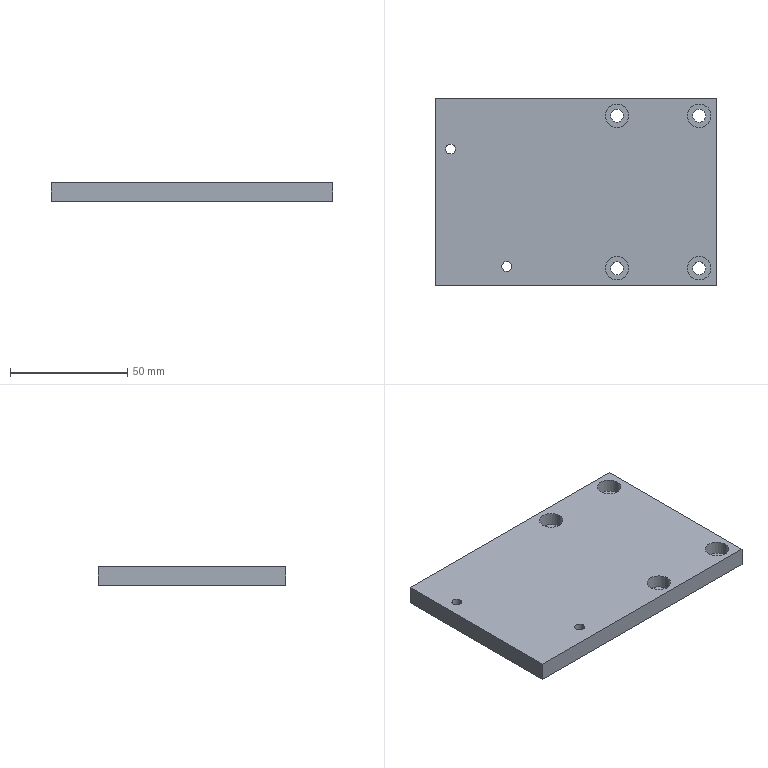Part | STEP file | X77-07006 | 1 solid | 30 faces | box 120 x 80 x 8 mm | volume 74569 mm3 | cylinder 20 | plane 10 | commonest cylinder face diameters 5.5 x8 10 x8 4.2 x4
STEP:
#1=CARTESIAN_POINT('',(-295.5,1019.962,2.3));
#2=VERTEX_POINT('',#1);
#3=CARTESIAN_POINT('',(-285.5,1019.962,2.3));
#4=VERTEX_POINT('',#3);
#5=CARTESIAN_POINT('',(-290.5,1019.962,2.3));
#6=DIRECTION('',(0.,0.,1.));
#7=DIRECTION('',(1.,0.,0.));
#8=AXIS2_PLACEMENT_3D('',#5,#6,#7);
#9=CIRCLE('',#8,5.);
#10=EDGE_CURVE('',#2,#4,#9,.T.);
#11=ORIENTED_EDGE('',*,*,#10,.F.);
#12=CARTESIAN_POINT('',(-295.5,1019.962,8.));
#13=VERTEX_POINT('',#12);
#14=CARTESIAN_POINT('',(-295.5,1019.962,8.));
#15=DIRECTION('',(0.,0.,1.));
#16=VECTOR('',#15,1000.);
#17=LINE('',#14,#16);
#18=EDGE_CURVE('',#2,#13,#17,.T.);
#19=ORIENTED_EDGE('',*,*,#18,.T.);
#20=CARTESIAN_POINT('',(-285.5,1019.962,8.));
#21=VERTEX_POINT('',#20);
#22=CARTESIAN_POINT('',(-290.5,1019.962,8.));
#23=DIRECTION('',(0.,0.,1.));
#24=DIRECTION('',(1.,0.,0.));
#25=AXIS2_PLACEMENT_3D('',#22,#23,#24);
#26=CIRCLE('',#25,5.);
#27=EDGE_CURVE('',#13,#21,#26,.T.);
#28=ORIENTED_EDGE('',*,*,#27,.T.);
#29=CARTESIAN_POINT('',(-285.5,1019.962,8.));
#30=DIRECTION('',(0.,0.,1.));
#31=VECTOR('',#30,1000.);
#32=LINE('',#29,#31);
#33=EDGE_CURVE('',#4,#21,#32,.T.);
#34=ORIENTED_EDGE('',*,*,#33,.F.);
#35=EDGE_LOOP('',(#11,#19,#28,#34));
#36=FACE_OUTER_BOUND('',#35,.T.);
#37=CARTESIAN_POINT('',(-290.5,1019.962,8.));
#38=DIRECTION('',(0.,0.,1.));
#39=DIRECTION('',(1.,0.,0.));
#40=AXIS2_PLACEMENT_3D('',#37,#38,#39);
#41=CYLINDRICAL_SURFACE('',#40,5.);
#42=ADVANCED_FACE('',(#36),#41,.F.);
#43=CARTESIAN_POINT('',(-293.25,1019.962,0.));
#44=VERTEX_POINT('',#43);
#45=CARTESIAN_POINT('',(-287.75,1019.962,0.));
#46=VERTEX_POINT('',#45);
#47=CARTESIAN_POINT('',(-290.5,1019.962,0.));
#48=DIRECTION('',(0.,0.,1.));
#49=DIRECTION('',(1.,0.,0.));
#50=AXIS2_PLACEMENT_3D('',#47,#48,#49);
#51=CIRCLE('',#50,2.75);
#52=EDGE_CURVE('',#44,#46,#51,.T.);
#53=ORIENTED_EDGE('',*,*,#52,.F.);
#54=CARTESIAN_POINT('',(-293.25,1019.962,2.3));
#55=VERTEX_POINT('',#54);
#56=CARTESIAN_POINT('',(-293.25,1019.962,8.));
#57=DIRECTION('',(0.,0.,1.));
#58=VECTOR('',#57,1000.);
#59=LINE('',#56,#58);
#60=EDGE_CURVE('',#44,#55,#59,.T.);
#61=ORIENTED_EDGE('',*,*,#60,.T.);
#62=CARTESIAN_POINT('',(-287.75,1019.962,2.3));
#63=VERTEX_POINT('',#62);
#64=CARTESIAN_POINT('',(-290.5,1019.962,2.3));
#65=DIRECTION('',(0.,0.,1.));
#66=DIRECTION('',(1.,0.,0.));
#67=AXIS2_PLACEMENT_3D('',#64,#65,#66);
#68=CIRCLE('',#67,2.75);
#69=EDGE_CURVE('',#55,#63,#68,.T.);
#70=ORIENTED_EDGE('',*,*,#69,.T.);
#71=CARTESIAN_POINT('',(-287.75,1019.962,8.));
#72=DIRECTION('',(0.,0.,1.));
#73=VECTOR('',#72,1000.);
#74=LINE('',#71,#73);
#75=EDGE_CURVE('',#46,#63,#74,.T.);
#76=ORIENTED_EDGE('',*,*,#75,.F.);
#77=EDGE_LOOP('',(#53,#61,#70,#76));
#78=FACE_OUTER_BOUND('',#77,.T.);
#79=CARTESIAN_POINT('',(-290.5,1019.962,8.));
#80=DIRECTION('',(0.,0.,1.));
#81=DIRECTION('',(1.,0.,0.));
#82=AXIS2_PLACEMENT_3D('',#79,#80,#81);
#83=CYLINDRICAL_SURFACE('',#82,2.75);
#84=ADVANCED_FACE('',(#78),#83,.F.);
#85=CARTESIAN_POINT('',(-260.5,1019.962,2.3));
#86=VERTEX_POINT('',#85);
#87=CARTESIAN_POINT('',(-250.5,1019.962,2.3));
#88=VERTEX_POINT('',#87);
#89=CARTESIAN_POINT('',(-255.5,1019.962,2.3));
#90=DIRECTION('',(0.,0.,1.));
#91=DIRECTION('',(1.,0.,0.));
#92=AXIS2_PLACEMENT_3D('',#89,#90,#91);
#93=CIRCLE('',#92,5.);
#94=EDGE_CURVE('',#86,#88,#93,.T.);
#95=ORIENTED_EDGE('',*,*,#94,.F.);
#96=CARTESIAN_POINT('',(-260.5,1019.962,8.));
#97=VERTEX_POINT('',#96);
#98=CARTESIAN_POINT('',(-260.5,1019.962,8.));
#99=DIRECTION('',(0.,0.,1.));
#100=VECTOR('',#99,1000.);
#101=LINE('',#98,#100);
#102=EDGE_CURVE('',#86,#97,#101,.T.);
#103=ORIENTED_EDGE('',*,*,#102,.T.);
#104=CARTESIAN_POINT('',(-250.5,1019.962,8.));
#105=VERTEX_POINT('',#104);
#106=CARTESIAN_POINT('',(-255.5,1019.962,8.));
#107=DIRECTION('',(0.,0.,1.));
#108=DIRECTION('',(1.,0.,0.));
#109=AXIS2_PLACEMENT_3D('',#106,#107,#108);
#110=CIRCLE('',#109,5.);
#111=EDGE_CURVE('',#97,#105,#110,.T.);
#112=ORIENTED_EDGE('',*,*,#111,.T.);
#113=CARTESIAN_POINT('',(-250.5,1019.962,8.));
#114=DIRECTION('',(0.,0.,1.));
#115=VECTOR('',#114,1000.);
#116=LINE('',#113,#115);
#117=EDGE_CURVE('',#88,#105,#116,.T.);
#118=ORIENTED_EDGE('',*,*,#117,.F.);
#119=EDGE_LOOP('',(#95,#103,#112,#118));
#120=FACE_OUTER_BOUND('',#119,.T.);
#121=CARTESIAN_POINT('',(-255.5,1019.962,8.));
#122=DIRECTION('',(0.,0.,1.));
#123=DIRECTION('',(1.,0.,0.));
#124=AXIS2_PLACEMENT_3D('',#121,#122,#123);
#125=CYLINDRICAL_SURFACE('',#124,5.);
#126=ADVANCED_FACE('',(#120),#125,.F.);
#127=CARTESIAN_POINT('',(-258.25,1019.962,0.));
#128=VERTEX_POINT('',#127);
#129=CARTESIAN_POINT('',(-252.75,1019.962,0.));
#130=VERTEX_POINT('',#129);
#131=CARTESIAN_POINT('',(-255.5,1019.962,0.));
#132=DIRECTION('',(0.,0.,1.));
#133=DIRECTION('',(1.,0.,0.));
#134=AXIS2_PLACEMENT_3D('',#131,#132,#133);
#135=CIRCLE('',#134,2.75);
#136=EDGE_CURVE('',#128,#130,#135,.T.);
#137=ORIENTED_EDGE('',*,*,#136,.F.);
#138=CARTESIAN_POINT('',(-258.25,1019.962,2.3));
#139=VERTEX_POINT('',#138);
#140=CARTESIAN_POINT('',(-258.25,1019.962,8.));
#141=DIRECTION('',(0.,0.,1.));
#142=VECTOR('',#141,1000.);
#143=LINE('',#140,#142);
#144=EDGE_CURVE('',#128,#139,#143,.T.);
#145=ORIENTED_EDGE('',*,*,#144,.T.);
#146=CARTESIAN_POINT('',(-252.75,1019.962,2.3));
#147=VERTEX_POINT('',#146);
#148=CARTESIAN_POINT('',(-255.5,1019.962,2.3));
#149=DIRECTION('',(0.,0.,1.));
#150=DIRECTION('',(1.,0.,0.));
#151=AXIS2_PLACEMENT_3D('',#148,#149,#150);
#152=CIRCLE('',#151,2.75);
#153=EDGE_CURVE('',#139,#147,#152,.T.);
#154=ORIENTED_EDGE('',*,*,#153,.T.);
#155=CARTESIAN_POINT('',(-252.75,1019.962,8.));
#156=DIRECTION('',(0.,0.,1.));
#157=VECTOR('',#156,1000.);
#158=LINE('',#155,#157);
#159=EDGE_CURVE('',#130,#147,#158,.T.);
#160=ORIENTED_EDGE('',*,*,#159,.F.);
#161=EDGE_LOOP('',(#137,#145,#154,#160));
#162=FACE_OUTER_BOUND('',#161,.T.);
#163=CARTESIAN_POINT('',(-255.5,1019.962,8.));
#164=DIRECTION('',(0.,0.,1.));
#165=DIRECTION('',(1.,0.,0.));
#166=AXIS2_PLACEMENT_3D('',#163,#164,#165);
#167=CYLINDRICAL_SURFACE('',#166,2.75);
#168=ADVANCED_FACE('',(#162),#167,.F.);
#169=CARTESIAN_POINT('',(-295.5,954.962,2.3));
#170=VERTEX_POINT('',#169);
#171=CARTESIAN_POINT('',(-285.5,954.962,2.3));
#172=VERTEX_POINT('',#171);
#173=CARTESIAN_POINT('',(-290.5,954.962,2.3));
#174=DIRECTION('',(0.,0.,1.));
#175=DIRECTION('',(1.,0.,0.));
#176=AXIS2_PLACEMENT_3D('',#173,#174,#175);
#177=CIRCLE('',#176,5.);
#178=EDGE_CURVE('',#170,#172,#177,.T.);
#179=ORIENTED_EDGE('',*,*,#178,.F.);
#180=CARTESIAN_POINT('',(-295.5,954.962,8.));
#181=VERTEX_POINT('',#180);
#182=CARTESIAN_POINT('',(-295.5,954.962,8.));
#183=DIRECTION('',(0.,0.,1.));
#184=VECTOR('',#183,1000.);
#185=LINE('',#182,#184);
#186=EDGE_CURVE('',#170,#181,#185,.T.);
#187=ORIENTED_EDGE('',*,*,#186,.T.);
#188=CARTESIAN_POINT('',(-285.5,954.962,8.));
#189=VERTEX_POINT('',#188);
#190=CARTESIAN_POINT('',(-290.5,954.962,8.));
#191=DIRECTION('',(0.,0.,1.));
#192=DIRECTION('',(1.,0.,0.));
#193=AXIS2_PLACEMENT_3D('',#190,#191,#192);
#194=CIRCLE('',#193,5.);
#195=EDGE_CURVE('',#181,#189,#194,.T.);
#196=ORIENTED_EDGE('',*,*,#195,.T.);
#197=CARTESIAN_POINT('',(-285.5,954.962,8.));
#198=DIRECTION('',(0.,0.,1.));
#199=VECTOR('',#198,1000.);
#200=LINE('',#197,#199);
#201=EDGE_CURVE('',#172,#189,#200,.T.);
#202=ORIENTED_EDGE('',*,*,#201,.F.);
#203=EDGE_LOOP('',(#179,#187,#196,#202));
#204=FACE_OUTER_BOUND('',#203,.T.);
#205=CARTESIAN_POINT('',(-290.5,954.962,8.));
#206=DIRECTION('',(0.,0.,1.));
#207=DIRECTION('',(1.,0.,0.));
#208=AXIS2_PLACEMENT_3D('',#205,#206,#207);
#209=CYLINDRICAL_SURFACE('',#208,5.);
#210=ADVANCED_FACE('',(#204),#209,.F.);
#211=CARTESIAN_POINT('',(-293.25,954.962,0.));
#212=VERTEX_POINT('',#211);
#213=CARTESIAN_POINT('',(-287.75,954.962,0.));
#214=VERTEX_POINT('',#213);
#215=CARTESIAN_POINT('',(-290.5,954.962,0.));
#216=DIRECTION('',(0.,0.,1.));
#217=DIRECTION('',(1.,0.,0.));
#218=AXIS2_PLACEMENT_3D('',#215,#216,#217);
#219=CIRCLE('',#218,2.75);
#220=EDGE_CURVE('',#212,#214,#219,.T.);
#221=ORIENTED_EDGE('',*,*,#220,.F.);
#222=CARTESIAN_POINT('',(-293.25,954.962,2.3));
#223=VERTEX_POINT('',#222);
#224=CARTESIAN_POINT('',(-293.25,954.962,8.));
#225=DIRECTION('',(0.,0.,1.));
#226=VECTOR('',#225,1000.);
#227=LINE('',#224,#226);
#228=EDGE_CURVE('',#212,#223,#227,.T.);
#229=ORIENTED_EDGE('',*,*,#228,.T.);
#230=CARTESIAN_POINT('',(-287.75,954.962,2.3));
#231=VERTEX_POINT('',#230);
#232=CARTESIAN_POINT('',(-290.5,954.962,2.3));
#233=DIRECTION('',(0.,0.,1.));
#234=DIRECTION('',(1.,0.,0.));
#235=AXIS2_PLACEMENT_3D('',#232,#233,#234);
#236=CIRCLE('',#235,2.75);
#237=EDGE_CURVE('',#223,#231,#236,.T.);
#238=ORIENTED_EDGE('',*,*,#237,.T.);
#239=CARTESIAN_POINT('',(-287.75,954.962,8.));
#240=DIRECTION('',(0.,0.,1.));
#241=VECTOR('',#240,1000.);
#242=LINE('',#239,#241);
#243=EDGE_CURVE('',#214,#231,#242,.T.);
#244=ORIENTED_EDGE('',*,*,#243,.F.);
#245=EDGE_LOOP('',(#221,#229,#238,#244));
#246=FACE_OUTER_BOUND('',#245,.T.);
#247=CARTESIAN_POINT('',(-290.5,954.962,8.));
#248=DIRECTION('',(0.,0.,1.));
#249=DIRECTION('',(1.,0.,0.));
#250=AXIS2_PLACEMENT_3D('',#247,#248,#249);
#251=CYLINDRICAL_SURFACE('',#250,2.75);
#252=ADVANCED_FACE('',(#246),#251,.F.);
#253=CARTESIAN_POINT('',(-260.5,954.962,2.3));
#254=VERTEX_POINT('',#253);
#255=CARTESIAN_POINT('',(-250.5,954.962,2.3));
#256=VERTEX_POINT('',#255);
#257=CARTESIAN_POINT('',(-255.5,954.962,2.3));
#258=DIRECTION('',(0.,0.,1.));
#259=DIRECTION('',(1.,0.,0.));
#260=AXIS2_PLACEMENT_3D('',#257,#258,#259);
#261=CIRCLE('',#260,5.);
#262=EDGE_CURVE('',#254,#256,#261,.T.);
#263=ORIENTED_EDGE('',*,*,#262,.F.);
#264=CARTESIAN_POINT('',(-260.5,954.962,8.));
#265=VERTEX_POINT('',#264);
#266=CARTESIAN_POINT('',(-260.5,954.962,8.));
#267=DIRECTION('',(0.,0.,1.));
#268=VECTOR('',#267,1000.);
#269=LINE('',#266,#268);
#270=EDGE_CURVE('',#254,#265,#269,.T.);
#271=ORIENTED_EDGE('',*,*,#270,.T.);
#272=CARTESIAN_POINT('',(-250.5,954.962,8.));
#273=VERTEX_POINT('',#272);
#274=CARTESIAN_POINT('',(-255.5,954.962,8.));
#275=DIRECTION('',(0.,0.,1.));
#276=DIRECTION('',(1.,0.,0.));
#277=AXIS2_PLACEMENT_3D('',#274,#275,#276);
#278=CIRCLE('',#277,5.);
#279=EDGE_CURVE('',#265,#273,#278,.T.);
#280=ORIENTED_EDGE('',*,*,#279,.T.);
#281=CARTESIAN_POINT('',(-250.5,954.962,8.));
#282=DIRECTION('',(0.,0.,1.));
#283=VECTOR('',#282,1000.);
#284=LINE('',#281,#283);
#285=EDGE_CURVE('',#256,#273,#284,.T.);
#286=ORIENTED_EDGE('',*,*,#285,.F.);
#287=EDGE_LOOP('',(#263,#271,#280,#286));
#288=FACE_OUTER_BOUND('',#287,.T.);
#289=CARTESIAN_POINT('',(-255.5,954.962,8.));
#290=DIRECTION('',(0.,0.,1.));
#291=DIRECTION('',(1.,0.,0.));
#292=AXIS2_PLACEMENT_3D('',#289,#290,#291);
#293=CYLINDRICAL_SURFACE('',#292,5.);
#294=ADVANCED_FACE('',(#288),#293,.F.);
#295=CARTESIAN_POINT('',(-258.25,954.962,0.));
#296=VERTEX_POINT('',#295);
#297=CARTESIAN_POINT('',(-252.75,954.962,0.));
#298=VERTEX_POINT('',#297);
#299=CARTESIAN_POINT('',(-255.5,954.962,0.));
#300=DIRECTION('',(0.,0.,1.));
#301=DIRECTION('',(1.,0.,0.));
#302=AXIS2_PLACEMENT_3D('',#299,#300,#301);
#303=CIRCLE('',#302,2.75);
#304=EDGE_CURVE('',#296,#298,#303,.T.);
#305=ORIENTED_EDGE('',*,*,#304,.F.);
#306=CARTESIAN_POINT('',(-258.25,954.962,2.3));
#307=VERTEX_POINT('',#306);
#308=CARTESIAN_POINT('',(-258.25,954.962,8.));
#309=DIRECTION('',(0.,0.,1.));
#310=VECTOR('',#309,1000.);
#311=LINE('',#308,#310);
#312=EDGE_CURVE('',#296,#307,#311,.T.);
#313=ORIENTED_EDGE('',*,*,#312,.T.);
#314=CARTESIAN_POINT('',(-252.75,954.962,2.3));
#315=VERTEX_POINT('',#314);
#316=CARTESIAN_POINT('',(-255.5,954.962,2.3));
#317=DIRECTION('',(0.,0.,1.));
#318=DIRECTION('',(1.,0.,0.));
#319=AXIS2_PLACEMENT_3D('',#316,#317,#318);
#320=CIRCLE('',#319,2.75);
#321=EDGE_CURVE('',#307,#315,#320,.T.);
#322=ORIENTED_EDGE('',*,*,#321,.T.);
#323=CARTESIAN_POINT('',(-252.75,954.962,8.));
#324=DIRECTION('',(0.,0.,1.));
#325=VECTOR('',#324,1000.);
#326=LINE('',#323,#325);
#327=EDGE_CURVE('',#298,#315,#326,.T.);
#328=ORIENTED_EDGE('',*,*,#327,.F.);
#329=EDGE_LOOP('',(#305,#313,#322,#328));
#330=FACE_OUTER_BOUND('',#329,.T.);
#331=CARTESIAN_POINT('',(-255.5,954.962,8.));
#332=DIRECTION('',(0.,0.,1.));
#333=DIRECTION('',(1.,0.,0.));
#334=AXIS2_PLACEMENT_3D('',#331,#332,#333);
#335=CYLINDRICAL_SURFACE('',#334,2.75);
#336=ADVANCED_FACE('',(#330),#335,.F.);
#337=CARTESIAN_POINT('',(-339.6,955.739,8.));
#338=VERTEX_POINT('',#337);
#339=CARTESIAN_POINT('',(-335.4,955.739,8.));
#340=VERTEX_POINT('',#339);
#341=CARTESIAN_POINT('',(-337.5,955.739,8.));
#342=DIRECTION('',(0.,0.,1.));
#343=DIRECTION('',(1.,0.,0.));
#344=AXIS2_PLACEMENT_3D('',#341,#342,#343);
#345=CIRCLE('',#344,2.1);
#346=EDGE_CURVE('',#338,#340,#345,.T.);
#347=ORIENTED_EDGE('',*,*,#346,.T.);
#348=CARTESIAN_POINT('',(-335.4,955.739,0.));
#349=VERTEX_POINT('',#348);
#350=CARTESIAN_POINT('',(-335.4,955.739,0.));
#351=DIRECTION('',(0.,0.,-1.));
#352=VECTOR('',#351,1000.);
#353=LINE('',#350,#352);
#354=EDGE_CURVE('',#340,#349,#353,.T.);
#355=ORIENTED_EDGE('',*,*,#354,.T.);
#356=CARTESIAN_POINT('',(-339.6,955.739,0.));
#357=VERTEX_POINT('',#356);
#358=CARTESIAN_POINT('',(-337.5,955.739,0.));
#359=DIRECTION('',(0.,0.,-1.));
#360=DIRECTION('',(-1.,0.,0.));
#361=AXIS2_PLACEMENT_3D('',#358,#359,#360);
#362=CIRCLE('',#361,2.1);
#363=EDGE_CURVE('',#349,#357,#362,.T.);
#364=ORIENTED_EDGE('',*,*,#363,.T.);
#365=CARTESIAN_POINT('',(-339.6,955.739,0.));
#366=DIRECTION('',(0.,0.,-1.));
#367=VECTOR('',#366,1000.);
#368=LINE('',#365,#367);
#369=EDGE_CURVE('',#338,#357,#368,.T.);
#370=ORIENTED_EDGE('',*,*,#369,.F.);
#371=EDGE_LOOP('',(#347,#355,#364,#370));
#372=FACE_OUTER_BOUND('',#371,.T.);
#373=CARTESIAN_POINT('',(-337.5,955.739,0.));
#374=DIRECTION('',(0.,0.,-1.));
#375=DIRECTION('',(-1.,0.,0.));
#376=AXIS2_PLACEMENT_3D('',#373,#374,#375);
#377=CYLINDRICAL_SURFACE('',#376,2.1);
#378=ADVANCED_FACE('',(#372),#377,.F.);
#379=CARTESIAN_POINT('',(-363.6,1005.739,8.));
#380=VERTEX_POINT('',#379);
#381=CARTESIAN_POINT('',(-359.4,1005.739,8.));
#382=VERTEX_POINT('',#381);
#383=CARTESIAN_POINT('',(-361.5,1005.739,8.));
#384=DIRECTION('',(0.,0.,1.));
#385=DIRECTION('',(1.,0.,0.));
#386=AXIS2_PLACEMENT_3D('',#383,#384,#385);
#387=CIRCLE('',#386,2.1);
#388=EDGE_CURVE('',#380,#382,#387,.T.);
#389=ORIENTED_EDGE('',*,*,#388,.T.);
#390=CARTESIAN_POINT('',(-359.4,1005.739,0.));
#391=VERTEX_POINT('',#390);
#392=CARTESIAN_POINT('',(-359.4,1005.739,0.));
#393=DIRECTION('',(0.,0.,-1.));
#394=VECTOR('',#393,1000.);
#395=LINE('',#392,#394);
#396=EDGE_CURVE('',#382,#391,#395,.T.);
#397=ORIENTED_EDGE('',*,*,#396,.T.);
#398=CARTESIAN_POINT('',(-363.6,1005.739,0.));
#399=VERTEX_POINT('',#398);
#400=CARTESIAN_POINT('',(-361.5,1005.739,0.));
#401=DIRECTION('',(0.,0.,-1.));
#402=DIRECTION('',(-1.,0.,0.));
#403=AXIS2_PLACEMENT_3D('',#400,#401,#402);
#404=CIRCLE('',#403,2.1);
#405=EDGE_CURVE('',#391,#399,#404,.T.);
#406=ORIENTED_EDGE('',*,*,#405,.T.);
#407=CARTESIAN_POINT('',(-363.6,1005.739,0.));
#408=DIRECTION('',(0.,0.,-1.));
#409=VECTOR('',#408,1000.);
#410=LINE('',#407,#409);
#411=EDGE_CURVE('',#380,#399,#410,.T.);
#412=ORIENTED_EDGE('',*,*,#411,.F.);
#413=EDGE_LOOP('',(#389,#397,#406,#412));
#414=FACE_OUTER_BOUND('',#413,.T.);
#415=CARTESIAN_POINT('',(-361.5,1005.739,0.));
#416=DIRECTION('',(0.,0.,-1.));
#417=DIRECTION('',(-1.,0.,0.));
#418=AXIS2_PLACEMENT_3D('',#415,#416,#417);
#419=CYLINDRICAL_SURFACE('',#418,2.1);
#420=ADVANCED_FACE('',(#414),#419,.F.);
#421=CARTESIAN_POINT('',(-368.,1027.462,0.));
#422=VERTEX_POINT('',#421);
#423=CARTESIAN_POINT('',(-368.,947.462,0.));
#424=VERTEX_POINT('',#423);
#425=CARTESIAN_POINT('',(-368.,1027.462,0.));
#426=DIRECTION('',(0.,-1.,0.));
#427=VECTOR('',#426,1000.);
#428=LINE('',#425,#427);
#429=EDGE_CURVE('',#422,#424,#428,.T.);
#430=ORIENTED_EDGE('',*,*,#429,.T.);
#431=CARTESIAN_POINT('',(-368.,947.462,8.));
#432=VERTEX_POINT('',#431);
#433=CARTESIAN_POINT('',(-368.,947.462,8.));
#434=DIRECTION('',(0.,0.,-1.));
#435=VECTOR('',#434,1000.);
#436=LINE('',#433,#435);
#437=EDGE_CURVE('',#432,#424,#436,.T.);
#438=ORIENTED_EDGE('',*,*,#437,.F.);
#439=CARTESIAN_POINT('',(-368.,1027.462,8.));
#440=VERTEX_POINT('',#439);
#441=CARTESIAN_POINT('',(-368.,1027.462,8.));
#442=DIRECTION('',(0.,-1.,0.));
#443=VECTOR('',#442,1000.);
#444=LINE('',#441,#443);
#445=EDGE_CURVE('',#440,#432,#444,.T.);
#446=ORIENTED_EDGE('',*,*,#445,.F.);
#447=CARTESIAN_POINT('',(-368.,1027.462,8.));
#448=DIRECTION('',(0.,0.,-1.));
#449=VECTOR('',#448,1000.);
#450=LINE('',#447,#449);
#451=EDGE_CURVE('',#440,#422,#450,.T.);
#452=ORIENTED_EDGE('',*,*,#451,.T.);
#453=EDGE_LOOP('',(#430,#438,#446,#452));
#454=FACE_OUTER_BOUND('',#453,.T.);
#455=CARTESIAN_POINT('',(-368.,1027.462,8.));
#456=DIRECTION('',(1.,0.,0.));
#457=DIRECTION('',(0.,0.,-1.));
#458=AXIS2_PLACEMENT_3D('',#455,#456,#457);
#459=PLANE('',#458);
#460=ADVANCED_FACE('',(#454),#459,.F.);
#461=CARTESIAN_POINT('',(-248.,947.462,0.));
#462=VERTEX_POINT('',#461);
#463=CARTESIAN_POINT('',(-368.,947.462,0.));
#464=DIRECTION('',(1.,0.,0.));
#465=VECTOR('',#464,1000.);
#466=LINE('',#463,#465);
#467=EDGE_CURVE('',#424,#462,#466,.T.);
#468=ORIENTED_EDGE('',*,*,#467,.T.);
#469=CARTESIAN_POINT('',(-248.,947.462,8.));
#470=VERTEX_POINT('',#469);
#471=CARTESIAN_POINT('',(-248.,947.462,8.));
#472=DIRECTION('',(0.,0.,-1.));
#473=VECTOR('',#472,1000.);
#474=LINE('',#471,#473);
#475=EDGE_CURVE('',#470,#462,#474,.T.);
#476=ORIENTED_EDGE('',*,*,#475,.F.);
#477=CARTESIAN_POINT('',(-368.,947.462,8.));
#478=DIRECTION('',(1.,0.,0.));
#479=VECTOR('',#478,1000.);
#480=LINE('',#477,#479);
#481=EDGE_CURVE('',#432,#470,#480,.T.);
#482=ORIENTED_EDGE('',*,*,#481,.F.);
#483=ORIENTED_EDGE('',*,*,#437,.T.);
#484=EDGE_LOOP('',(#468,#476,#482,#483));
#485=FACE_OUTER_BOUND('',#484,.T.);
#486=CARTESIAN_POINT('',(-368.,947.462,8.));
#487=DIRECTION('',(0.,1.,0.));
#488=DIRECTION('',(0.,0.,1.));
#489=AXIS2_PLACEMENT_3D('',#486,#487,#488);
#490=PLANE('',#489);
#491=ADVANCED_FACE('',(#485),#490,.F.);
#492=CARTESIAN_POINT('',(-248.,1027.462,0.));
#493=VERTEX_POINT('',#492);
#494=CARTESIAN_POINT('',(-248.,1027.462,0.));
#495=DIRECTION('',(0.,1.,0.));
#496=VECTOR('',#495,1000.);
#497=LINE('',#494,#496);
#498=EDGE_CURVE('',#462,#493,#497,.T.);
#499=ORIENTED_EDGE('',*,*,#498,.T.);
#500=CARTESIAN_POINT('',(-248.,1027.462,8.));
#501=VERTEX_POINT('',#500);
#502=CARTESIAN_POINT('',(-248.,1027.462,8.));
#503=DIRECTION('',(0.,0.,-1.));
#504=VECTOR('',#503,1000.);
#505=LINE('',#502,#504);
#506=EDGE_CURVE('',#501,#493,#505,.T.);
#507=ORIENTED_EDGE('',*,*,#506,.F.);
#508=CARTESIAN_POINT('',(-248.,1027.462,8.));
#509=DIRECTION('',(0.,1.,0.));
#510=VECTOR('',#509,1000.);
#511=LINE('',#508,#510);
#512=EDGE_CURVE('',#470,#501,#511,.T.);
#513=ORIENTED_EDGE('',*,*,#512,.F.);
#514=ORIENTED_EDGE('',*,*,#475,.T.);
#515=EDGE_LOOP('',(#499,#507,#513,#514));
#516=FACE_OUTER_BOUND('',#515,.T.);
#517=CARTESIAN_POINT('',(-248.,1027.462,8.));
#518=DIRECTION('',(-1.,0.,0.));
#519=DIRECTION('',(0.,-1.,0.));
#520=AXIS2_PLACEMENT_3D('',#517,#518,#519);
#521=PLANE('',#520);
#522=ADVANCED_FACE('',(#516),#521,.F.);
#523=CARTESIAN_POINT('',(-368.,1027.462,0.));
#524=DIRECTION('',(-1.,0.,0.));
#525=VECTOR('',#524,1000.);
#526=LINE('',#523,#525);
#527=EDGE_CURVE('',#493,#422,#526,.T.);
#528=ORIENTED_EDGE('',*,*,#527,.T.);
#529=ORIENTED_EDGE('',*,*,#451,.F.);
#530=CARTESIAN_POINT('',(-368.,1027.462,8.));
#531=DIRECTION('',(-1.,0.,0.));
#532=VECTOR('',#531,1000.);
#533=LINE('',#530,#532);
#534=EDGE_CURVE('',#501,#440,#533,.T.);
#535=ORIENTED_EDGE('',*,*,#534,.F.);
#536=ORIENTED_EDGE('',*,*,#506,.T.);
#537=EDGE_LOOP('',(#528,#529,#535,#536));
#538=FACE_OUTER_BOUND('',#537,.T.);
#539=CARTESIAN_POINT('',(-368.,1027.462,8.));
#540=DIRECTION('',(0.,-1.,0.));
#541=DIRECTION('',(0.,0.,-1.));
#542=AXIS2_PLACEMENT_3D('',#539,#540,#541);
#543=PLANE('',#542);
#544=ADVANCED_FACE('',(#538),#543,.F.);
#545=CARTESIAN_POINT('',(-290.5,1019.962,8.));
#546=DIRECTION('',(0.,0.,1.));
#547=DIRECTION('',(1.,0.,0.));
#548=AXIS2_PLACEMENT_3D('',#545,#546,#547);
#549=CIRCLE('',#548,5.);
#550=EDGE_CURVE('',#21,#13,#549,.T.);
#551=ORIENTED_EDGE('',*,*,#550,.F.);
#552=ORIENTED_EDGE('',*,*,#27,.F.);
#553=EDGE_LOOP('',(#551,#552));
#554=FACE_BOUND('',#553,.T.);
#555=CARTESIAN_POINT('',(-255.5,1019.962,8.));
#556=DIRECTION('',(0.,0.,1.));
#557=DIRECTION('',(1.,0.,0.));
#558=AXIS2_PLACEMENT_3D('',#555,#556,#557);
#559=CIRCLE('',#558,5.);
#560=EDGE_CURVE('',#105,#97,#559,.T.);
#561=ORIENTED_EDGE('',*,*,#560,.F.);
#562=ORIENTED_EDGE('',*,*,#111,.F.);
#563=EDGE_LOOP('',(#561,#562));
#564=FACE_BOUND('',#563,.T.);
#565=CARTESIAN_POINT('',(-290.5,954.962,8.));
#566=DIRECTION('',(0.,0.,1.));
#567=DIRECTION('',(1.,0.,0.));
#568=AXIS2_PLACEMENT_3D('',#565,#566,#567);
#569=CIRCLE('',#568,5.);
#570=EDGE_CURVE('',#189,#181,#569,.T.);
#571=ORIENTED_EDGE('',*,*,#570,.F.);
#572=ORIENTED_EDGE('',*,*,#195,.F.);
#573=EDGE_LOOP('',(#571,#572));
#574=FACE_BOUND('',#573,.T.);
#575=CARTESIAN_POINT('',(-255.5,954.962,8.));
#576=DIRECTION('',(0.,0.,1.));
#577=DIRECTION('',(1.,0.,0.));
#578=AXIS2_PLACEMENT_3D('',#575,#576,#577);
#579=CIRCLE('',#578,5.);
#580=EDGE_CURVE('',#273,#265,#579,.T.);
#581=ORIENTED_EDGE('',*,*,#580,.F.);
#582=ORIENTED_EDGE('',*,*,#279,.F.);
#583=EDGE_LOOP('',(#581,#582));
#584=FACE_BOUND('',#583,.T.);
#585=ORIENTED_EDGE('',*,*,#346,.F.);
#586=CARTESIAN_POINT('',(-337.5,955.739,8.));
#587=DIRECTION('',(0.,0.,1.));
#588=DIRECTION('',(1.,0.,0.));
#589=AXIS2_PLACEMENT_3D('',#586,#587,#588);
#590=CIRCLE('',#589,2.1);
#591=EDGE_CURVE('',#340,#338,#590,.T.);
#592=ORIENTED_EDGE('',*,*,#591,.F.);
#593=EDGE_LOOP('',(#585,#592));
#594=FACE_BOUND('',#593,.T.);
#595=ORIENTED_EDGE('',*,*,#388,.F.);
#596=CARTESIAN_POINT('',(-361.5,1005.739,8.));
#597=DIRECTION('',(0.,0.,1.));
#598=DIRECTION('',(1.,0.,0.));
#599=AXIS2_PLACEMENT_3D('',#596,#597,#598);
#600=CIRCLE('',#599,2.1);
#601=EDGE_CURVE('',#382,#380,#600,.T.);
#602=ORIENTED_EDGE('',*,*,#601,.F.);
#603=EDGE_LOOP('',(#595,#602));
#604=FACE_BOUND('',#603,.T.);
#605=ORIENTED_EDGE('',*,*,#445,.T.);
#606=ORIENTED_EDGE('',*,*,#481,.T.);
#607=ORIENTED_EDGE('',*,*,#512,.T.);
#608=ORIENTED_EDGE('',*,*,#534,.T.);
#609=EDGE_LOOP('',(#605,#606,#607,#608));
#610=FACE_OUTER_BOUND('',#609,.T.);
#611=CARTESIAN_POINT('',(-368.,947.462,8.));
#612=DIRECTION('',(0.,0.,1.));
#613=DIRECTION('',(1.,0.,0.));
#614=AXIS2_PLACEMENT_3D('',#611,#612,#613);
#615=PLANE('',#614);
#616=ADVANCED_FACE('',(#554,#564,#574,#584,#594,#604,#610),#615,.T.);
#617=CARTESIAN_POINT('',(-290.5,1019.962,0.));
#618=DIRECTION('',(0.,0.,1.));
#619=DIRECTION('',(1.,0.,0.));
#620=AXIS2_PLACEMENT_3D('',#617,#618,#619);
#621=CIRCLE('',#620,2.75);
#622=EDGE_CURVE('',#46,#44,#621,.T.);
#623=ORIENTED_EDGE('',*,*,#622,.T.);
#624=ORIENTED_EDGE('',*,*,#52,.T.);
#625=EDGE_LOOP('',(#623,#624));
#626=FACE_BOUND('',#625,.T.);
#627=CARTESIAN_POINT('',(-255.5,1019.962,0.));
#628=DIRECTION('',(0.,0.,1.));
#629=DIRECTION('',(1.,0.,0.));
#630=AXIS2_PLACEMENT_3D('',#627,#628,#629);
#631=CIRCLE('',#630,2.75);
#632=EDGE_CURVE('',#130,#128,#631,.T.);
#633=ORIENTED_EDGE('',*,*,#632,.T.);
#634=ORIENTED_EDGE('',*,*,#136,.T.);
#635=EDGE_LOOP('',(#633,#634));
#636=FACE_BOUND('',#635,.T.);
#637=CARTESIAN_POINT('',(-290.5,954.962,0.));
#638=DIRECTION('',(0.,0.,1.));
#639=DIRECTION('',(1.,0.,0.));
#640=AXIS2_PLACEMENT_3D('',#637,#638,#639);
#641=CIRCLE('',#640,2.75);
#642=EDGE_CURVE('',#214,#212,#641,.T.);
#643=ORIENTED_EDGE('',*,*,#642,.T.);
#644=ORIENTED_EDGE('',*,*,#220,.T.);
#645=EDGE_LOOP('',(#643,#644));
#646=FACE_BOUND('',#645,.T.);
#647=CARTESIAN_POINT('',(-255.5,954.962,0.));
#648=DIRECTION('',(0.,0.,1.));
#649=DIRECTION('',(1.,0.,0.));
#650=AXIS2_PLACEMENT_3D('',#647,#648,#649);
#651=CIRCLE('',#650,2.75);
#652=EDGE_CURVE('',#298,#296,#651,.T.);
#653=ORIENTED_EDGE('',*,*,#652,.T.);
#654=ORIENTED_EDGE('',*,*,#304,.T.);
#655=EDGE_LOOP('',(#653,#654));
#656=FACE_BOUND('',#655,.T.);
#657=CARTESIAN_POINT('',(-337.5,955.739,0.));
#658=DIRECTION('',(0.,0.,-1.));
#659=DIRECTION('',(-1.,0.,0.));
#660=AXIS2_PLACEMENT_3D('',#657,#658,#659);
#661=CIRCLE('',#660,2.1);
#662=EDGE_CURVE('',#357,#349,#661,.T.);
#663=ORIENTED_EDGE('',*,*,#662,.F.);
#664=ORIENTED_EDGE('',*,*,#363,.F.);
#665=EDGE_LOOP('',(#663,#664));
#666=FACE_BOUND('',#665,.T.);
#667=CARTESIAN_POINT('',(-361.5,1005.739,0.));
#668=DIRECTION('',(0.,0.,-1.));
#669=DIRECTION('',(-1.,0.,0.));
#670=AXIS2_PLACEMENT_3D('',#667,#668,#669);
#671=CIRCLE('',#670,2.1);
#672=EDGE_CURVE('',#399,#391,#671,.T.);
#673=ORIENTED_EDGE('',*,*,#672,.F.);
#674=ORIENTED_EDGE('',*,*,#405,.F.);
#675=EDGE_LOOP('',(#673,#674));
#676=FACE_BOUND('',#675,.T.);
#677=ORIENTED_EDGE('',*,*,#429,.F.);
#678=ORIENTED_EDGE('',*,*,#527,.F.);
#679=ORIENTED_EDGE('',*,*,#498,.F.);
#680=ORIENTED_EDGE('',*,*,#467,.F.);
#681=EDGE_LOOP('',(#677,#678,#679,#680));
#682=FACE_OUTER_BOUND('',#681,.T.);
#683=CARTESIAN_POINT('',(-368.,947.462,0.));
#684=DIRECTION('',(0.,0.,1.));
#685=DIRECTION('',(1.,0.,0.));
#686=AXIS2_PLACEMENT_3D('',#683,#684,#685);
#687=PLANE('',#686);
#688=ADVANCED_FACE('',(#626,#636,#646,#656,#666,#676,#682),#687,.F.);
#689=ORIENTED_EDGE('',*,*,#396,.F.);
#690=ORIENTED_EDGE('',*,*,#601,.T.);
#691=ORIENTED_EDGE('',*,*,#411,.T.);
#692=ORIENTED_EDGE('',*,*,#672,.T.);
#693=EDGE_LOOP('',(#689,#690,#691,#692));
#694=FACE_OUTER_BOUND('',#693,.T.);
#695=CARTESIAN_POINT('',(-361.5,1005.739,0.));
#696=DIRECTION('',(0.,0.,-1.));
#697=DIRECTION('',(-1.,0.,0.));
#698=AXIS2_PLACEMENT_3D('',#695,#696,#697);
#699=CYLINDRICAL_SURFACE('',#698,2.1);
#700=ADVANCED_FACE('',(#694),#699,.F.);
#701=ORIENTED_EDGE('',*,*,#354,.F.);
#702=ORIENTED_EDGE('',*,*,#591,.T.);
#703=ORIENTED_EDGE('',*,*,#369,.T.);
#704=ORIENTED_EDGE('',*,*,#662,.T.);
#705=EDGE_LOOP('',(#701,#702,#703,#704));
#706=FACE_OUTER_BOUND('',#705,.T.);
#707=CARTESIAN_POINT('',(-337.5,955.739,0.));
#708=DIRECTION('',(0.,0.,-1.));
#709=DIRECTION('',(-1.,0.,0.));
#710=AXIS2_PLACEMENT_3D('',#707,#708,#709);
#711=CYLINDRICAL_SURFACE('',#710,2.1);
#712=ADVANCED_FACE('',(#706),#711,.F.);
#713=ORIENTED_EDGE('',*,*,#312,.F.);
#714=ORIENTED_EDGE('',*,*,#652,.F.);
#715=ORIENTED_EDGE('',*,*,#327,.T.);
#716=CARTESIAN_POINT('',(-255.5,954.962,2.3));
#717=DIRECTION('',(0.,0.,1.));
#718=DIRECTION('',(1.,0.,0.));
#719=AXIS2_PLACEMENT_3D('',#716,#717,#718);
#720=CIRCLE('',#719,2.75);
#721=EDGE_CURVE('',#315,#307,#720,.T.);
#722=ORIENTED_EDGE('',*,*,#721,.T.);
#723=EDGE_LOOP('',(#713,#714,#715,#722));
#724=FACE_OUTER_BOUND('',#723,.T.);
#725=CARTESIAN_POINT('',(-255.5,954.962,8.));
#726=DIRECTION('',(0.,0.,1.));
#727=DIRECTION('',(1.,0.,0.));
#728=AXIS2_PLACEMENT_3D('',#725,#726,#727);
#729=CYLINDRICAL_SURFACE('',#728,2.75);
#730=ADVANCED_FACE('',(#724),#729,.F.);
#731=ORIENTED_EDGE('',*,*,#721,.F.);
#732=ORIENTED_EDGE('',*,*,#321,.F.);
#733=EDGE_LOOP('',(#731,#732));
#734=FACE_BOUND('',#733,.T.);
#735=CARTESIAN_POINT('',(-255.5,954.962,2.3));
#736=DIRECTION('',(0.,0.,1.));
#737=DIRECTION('',(1.,0.,0.));
#738=AXIS2_PLACEMENT_3D('',#735,#736,#737);
#739=CIRCLE('',#738,5.);
#740=EDGE_CURVE('',#256,#254,#739,.T.);
#741=ORIENTED_EDGE('',*,*,#740,.T.);
#742=ORIENTED_EDGE('',*,*,#262,.T.);
#743=EDGE_LOOP('',(#741,#742));
#744=FACE_OUTER_BOUND('',#743,.T.);
#745=CARTESIAN_POINT('',(-252.75,954.962,2.3));
#746=DIRECTION('',(0.,0.,-1.));
#747=DIRECTION('',(-1.,0.,0.));
#748=AXIS2_PLACEMENT_3D('',#745,#746,#747);
#749=PLANE('',#748);
#750=ADVANCED_FACE('',(#734,#744),#749,.F.);
#751=ORIENTED_EDGE('',*,*,#270,.F.);
#752=ORIENTED_EDGE('',*,*,#740,.F.);
#753=ORIENTED_EDGE('',*,*,#285,.T.);
#754=ORIENTED_EDGE('',*,*,#580,.T.);
#755=EDGE_LOOP('',(#751,#752,#753,#754));
#756=FACE_OUTER_BOUND('',#755,.T.);
#757=CARTESIAN_POINT('',(-255.5,954.962,8.));
#758=DIRECTION('',(0.,0.,1.));
#759=DIRECTION('',(1.,0.,0.));
#760=AXIS2_PLACEMENT_3D('',#757,#758,#759);
#761=CYLINDRICAL_SURFACE('',#760,5.);
#762=ADVANCED_FACE('',(#756),#761,.F.);
#763=ORIENTED_EDGE('',*,*,#228,.F.);
#764=ORIENTED_EDGE('',*,*,#642,.F.);
#765=ORIENTED_EDGE('',*,*,#243,.T.);
#766=CARTESIAN_POINT('',(-290.5,954.962,2.3));
#767=DIRECTION('',(0.,0.,1.));
#768=DIRECTION('',(1.,0.,0.));
#769=AXIS2_PLACEMENT_3D('',#766,#767,#768);
#770=CIRCLE('',#769,2.75);
#771=EDGE_CURVE('',#231,#223,#770,.T.);
#772=ORIENTED_EDGE('',*,*,#771,.T.);
#773=EDGE_LOOP('',(#763,#764,#765,#772));
#774=FACE_OUTER_BOUND('',#773,.T.);
#775=CARTESIAN_POINT('',(-290.5,954.962,8.));
#776=DIRECTION('',(0.,0.,1.));
#777=DIRECTION('',(1.,0.,0.));
#778=AXIS2_PLACEMENT_3D('',#775,#776,#777);
#779=CYLINDRICAL_SURFACE('',#778,2.75);
#780=ADVANCED_FACE('',(#774),#779,.F.);
#781=ORIENTED_EDGE('',*,*,#771,.F.);
#782=ORIENTED_EDGE('',*,*,#237,.F.);
#783=EDGE_LOOP('',(#781,#782));
#784=FACE_BOUND('',#783,.T.);
#785=CARTESIAN_POINT('',(-290.5,954.962,2.3));
#786=DIRECTION('',(0.,0.,1.));
#787=DIRECTION('',(1.,0.,0.));
#788=AXIS2_PLACEMENT_3D('',#785,#786,#787);
#789=CIRCLE('',#788,5.);
#790=EDGE_CURVE('',#172,#170,#789,.T.);
#791=ORIENTED_EDGE('',*,*,#790,.T.);
#792=ORIENTED_EDGE('',*,*,#178,.T.);
#793=EDGE_LOOP('',(#791,#792));
#794=FACE_OUTER_BOUND('',#793,.T.);
#795=CARTESIAN_POINT('',(-287.75,954.962,2.3));
#796=DIRECTION('',(0.,0.,-1.));
#797=DIRECTION('',(-1.,0.,0.));
#798=AXIS2_PLACEMENT_3D('',#795,#796,#797);
#799=PLANE('',#798);
#800=ADVANCED_FACE('',(#784,#794),#799,.F.);
#801=ORIENTED_EDGE('',*,*,#186,.F.);
#802=ORIENTED_EDGE('',*,*,#790,.F.);
#803=ORIENTED_EDGE('',*,*,#201,.T.);
#804=ORIENTED_EDGE('',*,*,#570,.T.);
#805=EDGE_LOOP('',(#801,#802,#803,#804));
#806=FACE_OUTER_BOUND('',#805,.T.);
#807=CARTESIAN_POINT('',(-290.5,954.962,8.));
#808=DIRECTION('',(0.,0.,1.));
#809=DIRECTION('',(1.,0.,0.));
#810=AXIS2_PLACEMENT_3D('',#807,#808,#809);
#811=CYLINDRICAL_SURFACE('',#810,5.);
#812=ADVANCED_FACE('',(#806),#811,.F.);
#813=ORIENTED_EDGE('',*,*,#144,.F.);
#814=ORIENTED_EDGE('',*,*,#632,.F.);
#815=ORIENTED_EDGE('',*,*,#159,.T.);
#816=CARTESIAN_POINT('',(-255.5,1019.962,2.3));
#817=DIRECTION('',(0.,0.,1.));
#818=DIRECTION('',(1.,0.,0.));
#819=AXIS2_PLACEMENT_3D('',#816,#817,#818);
#820=CIRCLE('',#819,2.75);
#821=EDGE_CURVE('',#147,#139,#820,.T.);
#822=ORIENTED_EDGE('',*,*,#821,.T.);
#823=EDGE_LOOP('',(#813,#814,#815,#822));
#824=FACE_OUTER_BOUND('',#823,.T.);
#825=CARTESIAN_POINT('',(-255.5,1019.962,8.));
#826=DIRECTION('',(0.,0.,1.));
#827=DIRECTION('',(1.,0.,0.));
#828=AXIS2_PLACEMENT_3D('',#825,#826,#827);
#829=CYLINDRICAL_SURFACE('',#828,2.75);
#830=ADVANCED_FACE('',(#824),#829,.F.);
#831=ORIENTED_EDGE('',*,*,#821,.F.);
#832=ORIENTED_EDGE('',*,*,#153,.F.);
#833=EDGE_LOOP('',(#831,#832));
#834=FACE_BOUND('',#833,.T.);
#835=CARTESIAN_POINT('',(-255.5,1019.962,2.3));
#836=DIRECTION('',(0.,0.,1.));
#837=DIRECTION('',(1.,0.,0.));
#838=AXIS2_PLACEMENT_3D('',#835,#836,#837);
#839=CIRCLE('',#838,5.);
#840=EDGE_CURVE('',#88,#86,#839,.T.);
#841=ORIENTED_EDGE('',*,*,#840,.T.);
#842=ORIENTED_EDGE('',*,*,#94,.T.);
#843=EDGE_LOOP('',(#841,#842));
#844=FACE_OUTER_BOUND('',#843,.T.);
#845=CARTESIAN_POINT('',(-252.75,1019.962,2.3));
#846=DIRECTION('',(0.,0.,-1.));
#847=DIRECTION('',(-1.,0.,0.));
#848=AXIS2_PLACEMENT_3D('',#845,#846,#847);
#849=PLANE('',#848);
#850=ADVANCED_FACE('',(#834,#844),#849,.F.);
#851=ORIENTED_EDGE('',*,*,#102,.F.);
#852=ORIENTED_EDGE('',*,*,#840,.F.);
#853=ORIENTED_EDGE('',*,*,#117,.T.);
#854=ORIENTED_EDGE('',*,*,#560,.T.);
#855=EDGE_LOOP('',(#851,#852,#853,#854));
#856=FACE_OUTER_BOUND('',#855,.T.);
#857=CARTESIAN_POINT('',(-255.5,1019.962,8.));
#858=DIRECTION('',(0.,0.,1.));
#859=DIRECTION('',(1.,0.,0.));
#860=AXIS2_PLACEMENT_3D('',#857,#858,#859);
#861=CYLINDRICAL_SURFACE('',#860,5.);
#862=ADVANCED_FACE('',(#856),#861,.F.);
#863=ORIENTED_EDGE('',*,*,#60,.F.);
#864=ORIENTED_EDGE('',*,*,#622,.F.);
#865=ORIENTED_EDGE('',*,*,#75,.T.);
#866=CARTESIAN_POINT('',(-290.5,1019.962,2.3));
#867=DIRECTION('',(0.,0.,1.));
#868=DIRECTION('',(1.,0.,0.));
#869=AXIS2_PLACEMENT_3D('',#866,#867,#868);
#870=CIRCLE('',#869,2.75);
#871=EDGE_CURVE('',#63,#55,#870,.T.);
#872=ORIENTED_EDGE('',*,*,#871,.T.);
#873=EDGE_LOOP('',(#863,#864,#865,#872));
#874=FACE_OUTER_BOUND('',#873,.T.);
#875=CARTESIAN_POINT('',(-290.5,1019.962,8.));
#876=DIRECTION('',(0.,0.,1.));
#877=DIRECTION('',(1.,0.,0.));
#878=AXIS2_PLACEMENT_3D('',#875,#876,#877);
#879=CYLINDRICAL_SURFACE('',#878,2.75);
#880=ADVANCED_FACE('',(#874),#879,.F.);
#881=ORIENTED_EDGE('',*,*,#871,.F.);
#882=ORIENTED_EDGE('',*,*,#69,.F.);
#883=EDGE_LOOP('',(#881,#882));
#884=FACE_BOUND('',#883,.T.);
#885=CARTESIAN_POINT('',(-290.5,1019.962,2.3));
#886=DIRECTION('',(0.,0.,1.));
#887=DIRECTION('',(1.,0.,0.));
#888=AXIS2_PLACEMENT_3D('',#885,#886,#887);
#889=CIRCLE('',#888,5.);
#890=EDGE_CURVE('',#4,#2,#889,.T.);
#891=ORIENTED_EDGE('',*,*,#890,.T.);
#892=ORIENTED_EDGE('',*,*,#10,.T.);
#893=EDGE_LOOP('',(#891,#892));
#894=FACE_OUTER_BOUND('',#893,.T.);
#895=CARTESIAN_POINT('',(-287.75,1019.962,2.3));
#896=DIRECTION('',(0.,0.,-1.));
#897=DIRECTION('',(-1.,0.,0.));
#898=AXIS2_PLACEMENT_3D('',#895,#896,#897);
#899=PLANE('',#898);
#900=ADVANCED_FACE('',(#884,#894),#899,.F.);
#901=ORIENTED_EDGE('',*,*,#18,.F.);
#902=ORIENTED_EDGE('',*,*,#890,.F.);
#903=ORIENTED_EDGE('',*,*,#33,.T.);
#904=ORIENTED_EDGE('',*,*,#550,.T.);
#905=EDGE_LOOP('',(#901,#902,#903,#904));
#906=FACE_OUTER_BOUND('',#905,.T.);
#907=CARTESIAN_POINT('',(-290.5,1019.962,8.));
#908=DIRECTION('',(0.,0.,1.));
#909=DIRECTION('',(1.,0.,0.));
#910=AXIS2_PLACEMENT_3D('',#907,#908,#909);
#911=CYLINDRICAL_SURFACE('',#910,5.);
#912=ADVANCED_FACE('',(#906),#911,.F.);
#913=CLOSED_SHELL('',(#42,#84,#126,#168,#210,#252,#294,#336,#378,#420,#460,#491,#522,#544,#616,#688,#700,#712,#730,#750,#762,#780,#800,#812,#830,#850,#862,#880,#900,#912));
#914=MANIFOLD_SOLID_BREP('',#913);
#915=CARTESIAN_POINT('',(0.,0.,0.));
#916=DIRECTION('',(0.,0.,1.));
#917=DIRECTION('',(1.,0.,0.));
#918=AXIS2_PLACEMENT_3D('',#915,#916,#917);
#919=(LENGTH_UNIT()NAMED_UNIT(*)SI_UNIT(.MILLI.,.METRE.));
#920=UNCERTAINTY_MEASURE_WITH_UNIT(LENGTH_MEASURE(0.00001),#919,'','');
#921=(NAMED_UNIT(*)PLANE_ANGLE_UNIT()SI_UNIT($,.RADIAN.));
#922=(NAMED_UNIT(*)SI_UNIT($,.STERADIAN.)SOLID_ANGLE_UNIT());
#923=(GEOMETRIC_REPRESENTATION_CONTEXT(3)GLOBAL_UNCERTAINTY_ASSIGNED_CONTEXT((#920))GLOBAL_UNIT_ASSIGNED_CONTEXT((#919,#921,#922))REPRESENTATION_CONTEXT('',''));
#924=ADVANCED_BREP_SHAPE_REPRESENTATION('',(#914,#918),#923);